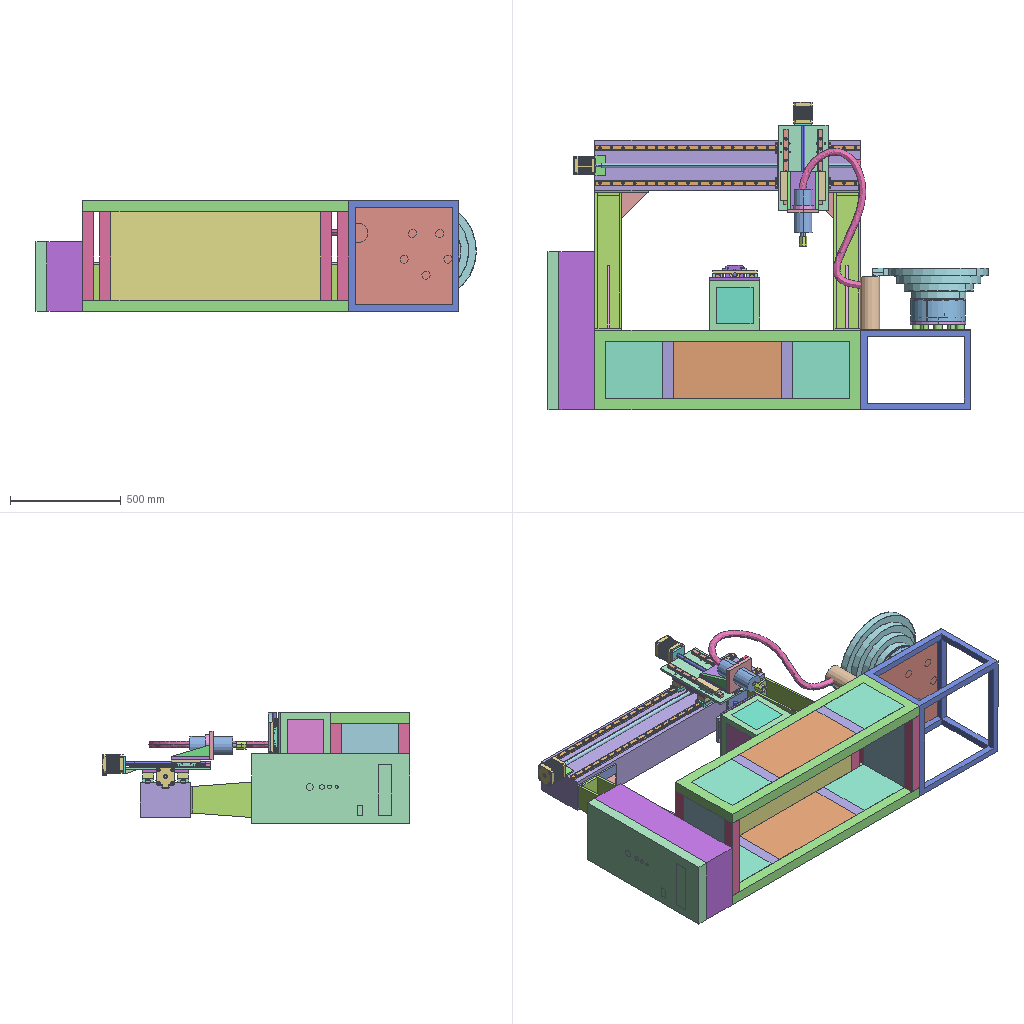Assembly | STEP file | 61 different items | 143 placed | box 1992 x 1390 x 500 mm
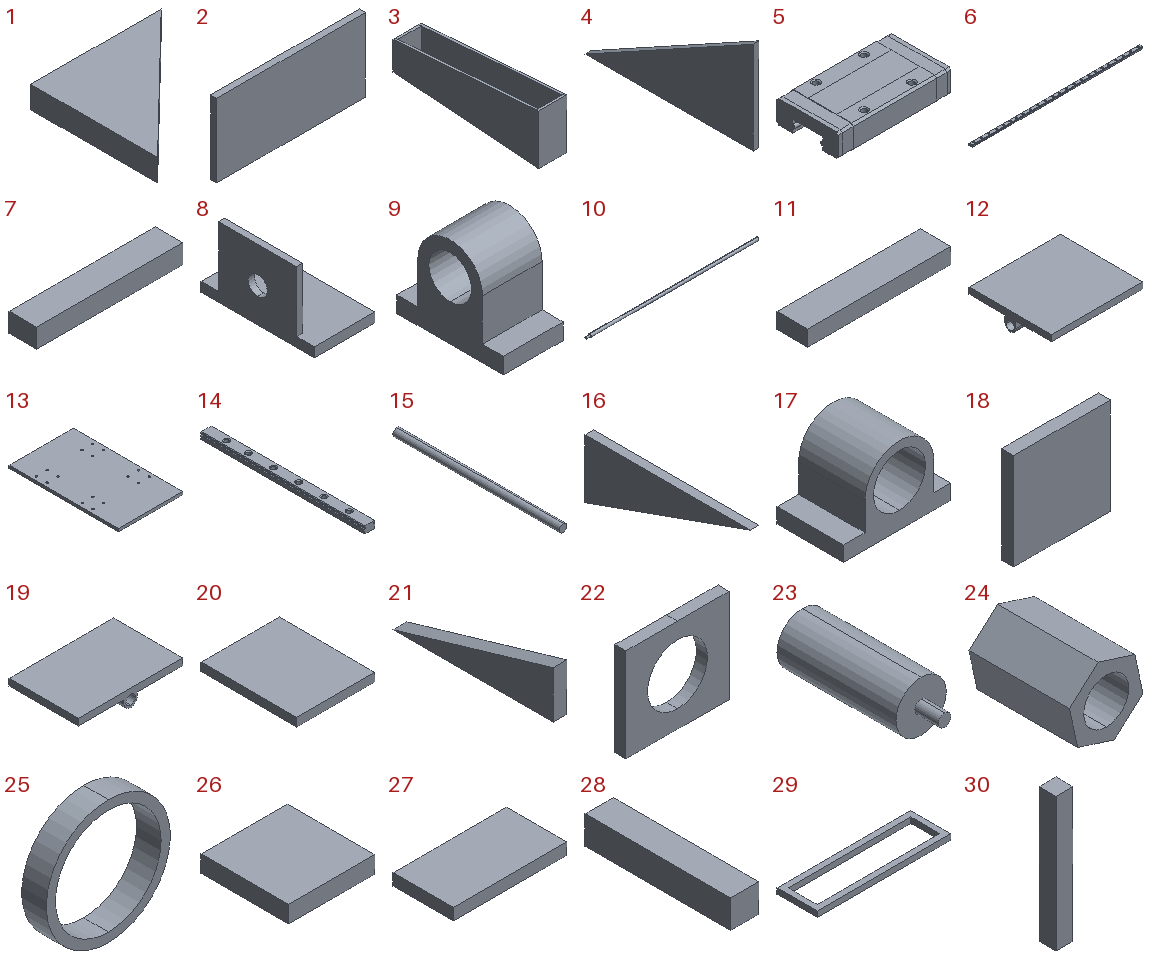Parts list (item | quantity | size | volume):
1 | x2 | 117.801 x 114.536 x 20 mm | 134925 mm3
2 | x2 | 243.554 x 10 x 120 mm | 292264 mm3
3 | x2 | 120 x 620.836 x 212.718 mm | 2999336 mm3
4 | x2 | 10 x 283.933 x 156.359 mm | 221977 mm3
5 | x8 | 88.2 x 48.75 x 18.375 mm | 58847 mm3
6 | x2 | 1200 x 22.5 x 15 mm | 367199 mm3
7 | x1 | 1200 x 227 x 156.72 mm | 9554357 mm3
8 | x1 | 48 x 90 x 55.597 mm | 46408 mm3
9 | x1 | 28 x 50 x 42.426 mm | 28637 mm3
10 | x1 | 1200 x 20 x 20 mm | 371431 mm3
11 | x2 | 229 x 49.201 x 25.123 mm | 283059 mm3
12 | x1 | 229 x 206.363 x 45.369 mm | 819761 mm3
13 | x1 | 225.075 x 384.491 x 10 mm | 860870 mm3
14 | x4 | 22.5 x 340 x 15 mm | 104637 mm3
15 | x2 | 18 x 384.491 x 18 mm | 97841 mm3
16 | x2 | 3 x 56.217 x 20 mm | 1687 mm3
17 | x1 | 37.23 x 23 x 26.824 mm | 9039 mm3
18 | x1 | 77.948 x 9.733 x 78 mm | 59173 mm3
19 | x2 | 200.887 x 133 x 32.213 mm | 365729 mm3
20 | x1 | 140.887 x 173 x 15 mm | 365603 mm3
21 | x2 | 15 x 173 x 50.952 mm | 66110 mm3
22 | x1 | 140.887 x 15 x 127.87 mm | 191936 mm3
23 | x1 | 81.521 x 231.5 x 81.521 mm | 1019717 mm3
24 | x1 | 32.935 x 45 x 33.783 mm | 20505 mm3
25 | x1 | 95.525 x 19 x 95.525 mm | 36998 mm3
26 | x4 | 255.311 x 259.164 x 50 mm | 3308367 mm3
27 | x2 | 489.379 x 259.164 x 50 mm | 6341468 mm3
28 | x4 | 50 x 259.164 x 50 mm | 647910 mm3
29 | x2 | 1200 x 359.164 x 50 mm | 7295820 mm3
30 | x6 | 50 x 50 x 400 mm | 1000000 mm3
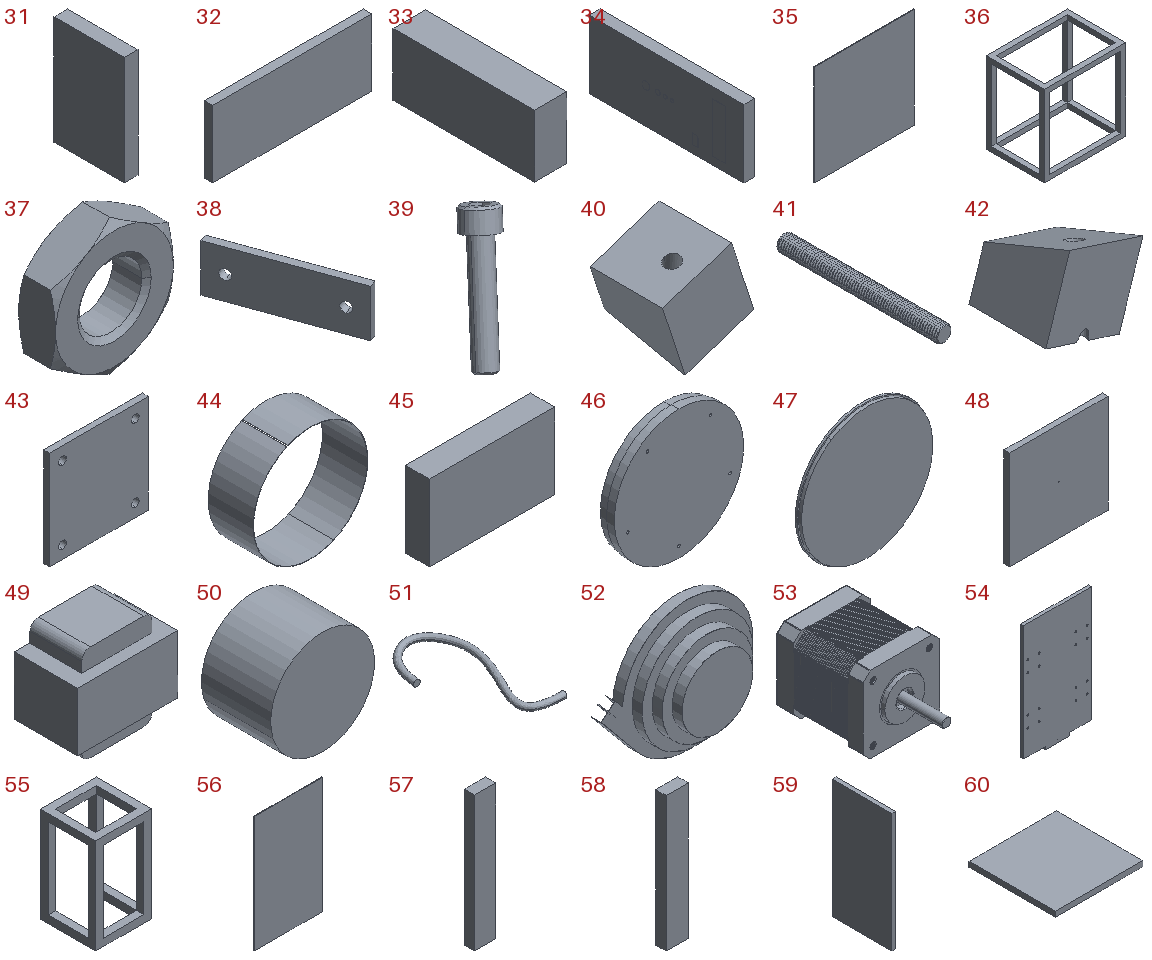31 | x2 | 50 x 259.164 x 400 mm | 5183281 mm3
32 | x1 | 947.9 x 50 x 400 mm | 18958001 mm3
33 | x1 | 162.496 x 714.237 x 313.918 mm | 36433685 mm3
34 | x1 | 51.504 x 714.237 x 313.918 mm | 11131790 mm3
35 | x1 | 498.959 x 2 x 500 mm | 498959 mm3
36 | x1 | 498.959 x 359.164 x 500 mm | 4457242 mm3
37 | x12 | 7.84 x 2.45 x 9.053 mm | 94.615 mm3
38 | x10 | 27.146 x 65.804 x 24.5 mm | 6425 mm3
39 | x10 | 14.373 x 15.735 x 28.731 mm | 656.353 mm3
40 | x5 | 30.872 x 24.5 x 30.872 mm | 11634 mm3
41 | x4 | 4.9 x 49 x 4.9 mm | 811.939 mm3
42 | x5 | 30.872 x 24.5 x 30.872 mm | 11423 mm3
43 | x1 | 66.15 x 3.92 x 66.15 mm | 16827 mm3
44 | x1 | 246.568 x 97.02 x 246.568 mm | 58546 mm3
45 | x1 | 58.8 x 11.27 x 35.77 mm | 23704 mm3
46 | x1 | 249.9 x 29.4 x 249.9 mm | 1411943 mm3
47 | x1 | 249.9 x 9.8 x 249.9 mm | 469473 mm3
48 | x1 | 61.25 x 3.43 x 61.25 mm | 12867 mm3
49 | x1 | 58.8 x 37.24 x 56.35 mm | 101666 mm3
50 | x5 | 36.75 x 34.3 x 36.75 mm | 26254 mm3
51 | x1 | 324.826 x 634.125 x 30 mm | 760478 mm3
52 | x1 | 524.053 x 137.2 x 450.8 mm | 389951 mm3
53 | x3 | 84 x 145 x 94 mm | 649991 mm3
54 | x1 | 225.075 x 66.921 x 394.223 mm | 895884 mm3
55 | x1 | 226.259 x 224 x 387.57 mm | 2434549 mm3
56 | x1 | 226.259 x 2 x 387.57 mm | 175382 mm3
57 | x1 | 20.737 x 10 x 133 mm | 27580 mm3
58 | x1 | 21.772 x 10 x 133 mm | 28956 mm3
59 | x2 | 10 x 164 x 327.57 mm | 537214 mm3
60 | x2 | 166.259 x 164 x 10 mm | 272664 mm3
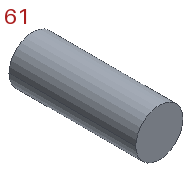61 | x1 | 89.417 x 240 x 89.417 mm | 636634 mm3
Placements (level | parent | child | x y z in mm | rotation matrix by rows):
1 | subassembly 2 | subassembly 3 | -0.0 -0.0 -0.0 | 1 0 0 0 1 0 0 0 1
1 | subassembly 2 | subassembly 3 | -0.0 -0.0 -0.0 | -1 0 0 0 1 0 0 0 -1
1 | subassembly 2 | subassembly 4 | -0.0 -0.0 -0.0 | 1 0 0 0 1 0 0 0 1
1 | subassembly 2 | subassembly 4 | 0.0 870.0 0.0 | -1 0 0 0 -1 0 0 0 1
1 | subassembly 2 | subassembly 5 | -0.0 -0.0 -0.0 | 1 0 0 0 1 0 0 0 1
1 | subassembly 2 | subassembly 5 | 1080.0 -0.0 -0.0 | 1 0 0 0 1 0 0 0 1
1 | subassembly 2 | subassembly 6 | -0.0 -0.0 -0.0 | 1 0 0 0 1 0 0 0 1
1 | subassembly 2 | subassembly 6 | 1077.681 0.0 0.0 | 1 0 0 0 1 0 0 0 1
1 | subassembly 2 | subassembly 7 | -0.0 -0.0 -0.0 | 1 0 0 0 1 0 0 0 1
1 | subassembly 2 | subassembly 7 | 841.273 1107.0 -0.0 | -1 0 0 0 -1 0 0 0 1
1 | subassembly 2 | subassembly 7 | -159.975 -0.0 -0.0 | 1 0 0 0 1 0 0 0 1
1 | subassembly 2 | subassembly 7 | 681.297 1107.0 -0.0 | -1 0 0 0 -1 0 0 0 1
1 | subassembly 2 | subassembly 7 | 896.886 38.582 71.806 | 0 -1 0 1 0 0 0 0 1
1 | subassembly 2 | subassembly 7 | -215.589 879.855 71.806 | 0 1 0 -1 0 0 0 0 1
1 | subassembly 2 | subassembly 7 | 588.111 -30.042 705.358 | 0 -1 0 0 0 1 -1 0 -0
1 | subassembly 2 | subassembly 7 | -524.365 -30.042 -135.915 | 0 1 0 0 0 1 1 0 -0
1 | subassembly 2 | subassembly 8 | -0.0 -0.0 -0.0 | 1 0 0 0 1 0 0 0 1
1 | subassembly 2 | subassembly 8 | -0.0 1107.0 -0.0 | -1 0 0 0 -1 0 0 0 1
1 | subassembly 2 | subassembly 9 | -0.0 -0.0 -0.0 | 1 0 0 0 1 0 0 0 1
1 | subassembly 2 | subassembly 10 | -0.0 -0.0 -0.0 | 1 0 0 0 1 0 0 0 1
1 | subassembly 2 | subassembly 11 | -0.0 -0.0 -0.0 | 1 0 0 0 1 0 0 0 1
1 | subassembly 2 | subassembly 12 | -0.0 -0.0 -0.0 | 1 0 0 0 1 0 0 0 1
1 | subassembly 2 | subassembly 13 | -0.0 -0.0 -0.0 | 1 0 0 0 1 0 0 0 1
1 | subassembly 2 | subassembly 13 | -0.0 157.162 -0.0 | 1 0 0 0 1 0 0 0 1
1 | subassembly 2 | subassembly 14 | -0.0 -0.0 -0.0 | 1 0 0 0 1 0 0 0 1
1 | subassembly 2 | subassembly 15 | -0.0 -0.0 -0.0 | 1 0 0 0 1 0 0 0 1
1 | subassembly 2 | subassembly 16 | -0.0 -0.0 -0.0 | 1 0 0 0 1 0 0 0 1
1 | subassembly 2 | subassembly 16 | 155.137 -0.0 0.0 | 1 0 0 0 1 0 0 0 1
1 | subassembly 2 | subassembly 16 | -308.776 -101.849 743.94 | 1 0 0 0 0 1 0 -1 0
1 | subassembly 2 | subassembly 16 | -153.638 -101.849 743.94 | 1 0 0 0 0 1 0 -1 -0
1 | subassembly 2 | subassembly 17 | -0.0 -0.0 -0.0 | 1 0 0 0 1 0 0 0 1
1 | subassembly 2 | subassembly 17 | 372.522 222.018 743.94 | -1 0 0 0 0 -1 0 -1 0
1 | subassembly 2 | subassembly 18 | -0.0 -0.0 -0.0 | 1 0 0 0 1 0 0 0 1
1 | subassembly 2 | subassembly 18 | -44.948 0.0 -0.0 | 1 0 0 0 1 0 0 0 1
1 | subassembly 2 | subassembly 19 | -0.0 -0.0 -0.0 | 1 0 0 0 1 0 0 0 1
1 | subassembly 2 | subassembly 20 | -0.0 -0.0 -0.0 | 1 0 0 0 1 0 0 0 1
1 | subassembly 2 | subassembly 21 | -0.0 -0.0 -0.0 | 1 0 0 0 1 0 0 0 1
1 | subassembly 2 | subassembly 21 | -308.776 -101.849 743.94 | 1 0 0 0 0 1 0 -1 0
1 | subassembly 2 | subassembly 22 | -0.0 -0.0 -0.0 | 1 0 0 0 1 0 0 0 1
1 | subassembly 2 | subassembly 23 | -0.0 -0.0 -0.0 | 1 0 0 0 1 0 0 0 1
1 | subassembly 2 | subassembly 23 | 125.887 -0.0 0.0 | 1 0 0 0 1 0 0 0 1
1 | subassembly 2 | subassembly 24 | -0.0 -0.0 -0.0 | 1 0 0 0 1 0 0 0 1
1 | subassembly 2 | subassembly 25 | -0.0 -0.0 -0.0 | 1 0 0 0 1 0 0 0 1
1 | subassembly 2 | subassembly 26 | -0.0 -0.0 -0.0 | 1 0 0 0 1 0 0 0 1
1 | subassembly 2 | subassembly 27 | -0.0 -0.0 -0.0 | 1 0 0 0 1 0 0 0 1
1 | subassembly 2 | subassembly 28 | -0.0 -0.0 -0.0 | 1 0 0 0 1 0 0 0 1
1 | subassembly 2 | subassembly 28 | 844.689 -0.0 -0.0 | 1 0 0 0 1 0 0 0 1
1 | subassembly 2 | subassembly 28 | 844.689 -0.0 -450.0 | 1 0 0 0 1 0 0 0 1
1 | subassembly 2 | subassembly 28 | -0.0 -0.0 -450.0 | 1 0 0 0 1 0 0 0 1
1 | subassembly 2 | subassembly 29 | -0.0 -0.0 -0.0 | 1 0 0 0 1 0 0 0 1
1 | subassembly 2 | subassembly 29 | -0.0 -0.0 -450.0 | 1 0 0 0 1 0 0 0 1
1 | subassembly 2 | subassembly 30 | -0.0 -0.0 -0.0 | 1 0 0 0 1 0 0 0 1
1 | subassembly 2 | subassembly 30 | 0.0 -0.0 737.282 | -1 0 0 0 1 0 0 0 -1
1 | subassembly 2 | subassembly 30 | -0.0 -0.0 -450.0 | 1 0 0 0 1 0 0 0 1
1 | subassembly 2 | subassembly 30 | 0.0 0.0 287.282 | -1 0 0 0 1 0 0 0 -1
1 | subassembly 2 | subassembly 31 | -0.0 -0.0 -0.0 | 1 0 0 0 1 0 0 0 1
1 | subassembly 2 | subassembly 31 | 0.0 0.0 -450.0 | 1 0 0 0 1 0 0 0 1
1 | subassembly 2 | subassembly 32 | -0.0 -0.0 -0.0 | 1 0 0 0 1 0 0 0 1
1 | subassembly 2 | subassembly 32 | -76.05 -0.0 -0.0 | 1 0 0 0 1 0 0 0 1
1 | subassembly 2 | subassembly 32 | -76.05 -309.164 -0.0 | 1 0 0 0 1 0 0 0 1
1 | subassembly 2 | subassembly 32 | 997.9 0.0 -0.0 | 1 0 0 0 1 0 0 0 1
1 | subassembly 2 | subassembly 32 | 1073.95 0.0 -0.0 | 1 0 0 0 1 0 0 0 1
1 | subassembly 2 | subassembly 32 | 76.05 -309.164 287.282 | -1 0 0 0 1 0 0 0 -1
1 | subassembly 2 | subassembly 33 | -0.0 -0.0 -0.0 | 1 0 0 0 1 0 0 0 1
1 | subassembly 2 | subassembly 33 | 1150.0 0.0 0.0 | 1 0 0 0 1 0 0 0 1
1 | subassembly 2 | subassembly 34 | -0.0 -0.0 -0.0 | 1 0 0 0 1 0 0 0 1
1 | subassembly 2 | subassembly 35 | -0.0 -0.0 -0.0 | 1 0 0 0 1 0 0 0 1
1 | subassembly 2 | subassembly 36 | -0.0 -0.0 -0.0 | 1 0 0 0 1 0 0 0 1
1 | subassembly 2 | subassembly 37 | -0.0 -0.0 -0.0 | 1 0 0 0 1 0 0 0 1
1 | subassembly 2 | subassembly 38 | -0.0 -0.0 -0.0 | 1 0 0 0 1 0 0 0 1
1 | subassembly 2 | subassembly 39 | -0.0 -0.0 -0.0 | 1 0 0 0 1 0 0 0 1
1 | subassembly 2 | subassembly 39 | 0.0001 -6.37 48.999 | 1 0 0 0 1 0 0 0 1
1 | subassembly 2 | subassembly 39 | -49.0 -6.37 -0.0001 | 1 0 0 0 1 0 0 0 1
1 | subassembly 2 | subassembly 39 | -49.0 -23.462 49 | 1 0 0 0 1 0 0 0 1
1 | subassembly 2 | subassembly 39 | -49 0.0 48.999 | 1 0 -1e-06 0 1 0 1e-06 0 1
1 | subassembly 2 | subassembly 39 | -49 -6.37 49.001 | 1 0 0 0 1 0 0 0 1
1 | subassembly 2 | subassembly 39 | 0.0 -23.462 -0.0001 | 1 0 0 0 1 0 0 0 1
1 | subassembly 2 | subassembly 39 | -49.0 -23.462 -0.0002 | 1 0 0 0 1 0 0 0 1
1 | subassembly 2 | subassembly 39 | 0.0 -23.462 49.0 | 1 0 0 0 1 0 0 0 1
1 | subassembly 2 | subassembly 39 | 0.0 -6.37 -0.0 | 1 0 0 0 1 0 0 0 1
1 | subassembly 2 | subassembly 39 | -49.0 0.0 0.0001 | 1 0 0 0 1 0 0 0 1
1 | subassembly 2 | subassembly 39 | 0.0 -0.0 49 | 1 0 0 0 1 0 0 0 1
1 | subassembly 2 | subassembly 40 | -0.0 -0.0 -0.0 | 1 0 0 0 1 0 0 0 1
1 | subassembly 2 | subassembly 40 | 808.883 -1.676 -796.145 | 0.309 0 -0.9511 0 1 0 0.9511 0 0.309
1 | subassembly 2 | subassembly 40 | 502.616 -0.0 1015.316 | 0.309 0 0.9511 0 1 0 -0.9511 0 0.309
1 | subassembly 2 | subassembly 40 | 1813.718 -0.0 -265.789 | -0.809 0 -0.5878 0 1 0 0.5878 0 -0.809
1 | subassembly 2 | subassembly 40 | 1817.444 -1.676 -268.495 | -0.809 0 -0.5878 0 1 0 0.5878 0 -0.809
1 | subassembly 2 | subassembly 40 | 1623.556 -0.0 851.049 | -0.809 0 0.5878 0 1 0 -0.5878 0 -0.809
1 | subassembly 2 | subassembly 40 | 1627.281 -1.676 853.756 | -0.809 0 0.5878 0 1 0 -0.5878 0 -0.809
1 | subassembly 2 | subassembly 40 | -4.604 -1.676 -0.0 | 1 0 0 0 1 0 0 0 1
1 | subassembly 2 | subassembly 40 | 810.306 -0.0 -791.766 | 0.309 0 -0.9511 0 1 0 0.9511 0 0.309
1 | subassembly 2 | subassembly 40 | 501.193 -1.676 1019.695 | 0.309 0 0.9511 0 1 0 -0.9511 0 0.309
1 | subassembly 2 | subassembly 41 | -0.0 -0.0 -0.0 | 1 0 0 0 1 0 0 0 1
1 | subassembly 2 | subassembly 41 | 1057.854 -661.138 -476.93 | -0.1707 -0.9797 0.1055 0.7998 -0.2002 -0.5659 0.5755 -0.01224 0.8177
1 | subassembly 2 | subassembly 41 | 362.365 -707.182 -147.994 | 0.4946 -0.3144 0.8102 0.7998 -0.2002 -0.5659 0.3402 0.9279 0.1524
1 | subassembly 2 | subassembly 41 | 485.857 46.045 1015.316 | 0.309 0 0.9511 0 1 0 -0.9511 0 0.309
1 | subassembly 2 | subassembly 41 | 487.401 -661.138 615.103 | 0.4764 0.7854 0.3953 0.7998 -0.2002 -0.5659 -0.3653 0.5857 -0.7235
1 | subassembly 2 | subassembly 41 | 375.924 -661.138 -138.143 | 0.4946 -0.3144 0.8102 0.7998 -0.2002 -0.5659 0.3402 0.9279 0.1524
1 | subassembly 2 | subassembly 41 | 502.616 -0.0 1015.316 | 0.309 0 0.9511 0 1 0 -0.9511 0 0.309
1 | subassembly 2 | subassembly 41 | -5.179 46.045 -15.939 | 1 0 0 0 1 0 0 0 1
1 | subassembly 2 | subassembly 41 | 1063.033 -707.182 -492.869 | -0.1707 -0.9797 0.1055 0.7998 -0.2002 -0.5659 0.5755 -0.01224 0.8177
1 | subassembly 2 | subassembly 41 | 473.843 -707.182 624.953 | 0.4764 0.7854 0.3953 0.7998 -0.2002 -0.5659 -0.3653 0.5857 -0.7235
1 | subassembly 2 | subassembly 42 | -0.0 -0.0 -0.0 | 1 0 0 0 1 0 0 0 1
1 | subassembly 2 | subassembly 42 | 810.306 -0.0 -791.766 | 0.309 0 -0.9511 0 1 0 0.9511 0 0.309
1 | subassembly 2 | subassembly 42 | 1813.718 0.0 -265.789 | -0.809 0 -0.5878 0 1 0 0.5878 0 -0.809
1 | subassembly 2 | subassembly 42 | 502.616 -0.0 1015.316 | 0.309 0 0.9511 0 1 0 -0.9511 0 0.309
1 | subassembly 2 | subassembly 42 | 1623.556 -0.0 851.049 | -0.809 0 0.5878 0 1 0 -0.5878 0 -0.809
1 | subassembly 2 | subassembly 43 | -0.0 -0.0 -0.0 | 1 0 0 0 1 0 0 0 1
1 | subassembly 2 | subassembly 43 | -49.0 0.0 -49.0 | 1 0 0 0 1 0 0 0 1
1 | subassembly 2 | subassembly 43 | -0.0 -0.0 -49.0 | 1 0 0 0 1 0 0 0 1
1 | subassembly 2 | subassembly 43 | -49.0 0.0 -0.0 | 1 0 0 0 1 0 0 0 1
1 | subassembly 2 | subassembly 44 | -0.0 -0.0 -0.0 | 1 0 0 0 1 0 0 0 1
1 | subassembly 2 | subassembly 44 | 502.616 -0.0 1015.316 | 0.309 0 0.9511 0 1 0 -0.9511 0 0.309
1 | subassembly 2 | subassembly 44 | 1623.556 -0.0 851.049 | -0.809 0 0.5878 0 1 0 -0.5878 0 -0.809
1 | subassembly 2 | subassembly 44 | 810.306 -0.0 -791.766 | 0.309 0 -0.9511 0 1 0 0.9511 0 0.309
1 | subassembly 2 | subassembly 44 | 1813.718 -0.0 -265.789 | -0.809 0 -0.5878 0 1 0 0.5878 0 -0.809
1 | subassembly 2 | subassembly 45 | -0.0 -0.0 -0.0 | 1 0 0 0 1 0 0 0 1
1 | subassembly 2 | subassembly 46 | -0.0 -0.0 -0.0 | 1 0 0 0 1 0 0 0 1
1 | subassembly 2 | subassembly 47 | -0.0 -0.0 -0.0 | 1 0 0 0 1 0 0 0 1
1 | subassembly 2 | subassembly 48 | -0.0 -0.0 -0.0 | 1 0 0 0 1 0 0 0 1
1 | subassembly 2 | subassembly 49 | -0.0 -0.0 -0.0 | 1 0 0 0 1 0 0 0 1
1 | subassembly 2 | subassembly 50 | -0.0 -0.0 -0.0 | 1 0 0 0 1 0 0 0 1
1 | subassembly 2 | subassembly 51 | -0.0 -0.0 -0.0 | 1 0 0 0 1 0 0 0 1
1 | subassembly 2 | subassembly 52 | -0.0 -0.0 -0.0 | 1 0 0 0 1 0 0 0 1
1 | subassembly 2 | subassembly 52 | 759.25 -0.0 1097.011 | 0 0 1 0 1 0 -1 0 -0
1 | subassembly 2 | subassembly 52 | 99.029 -0.0 -71.949 | 1 0 0 0 1 0 0 0 1
1 | subassembly 2 | subassembly 52 | 881.657 0.0 1097.011 | 0 0 1 0 1 0 -1 0 -0
1 | subassembly 2 | subassembly 52 | 198.058 -0.0 -0.0 | 1 0 0 0 1 0 0 0 1
1 | subassembly 2 | subassembly 53 | -0.0 -0.0 -0.0 | 1 0 0 0 1 0 0 0 1
1 | subassembly 2 | subassembly 54 | -0.0 -0.0 -0.0 | 1 0 0 0 1 0 0 0 1
1 | subassembly 2 | subassembly 55 | -0.0 -0.0 -0.0 | 1 0 0 0 1 0 0 0 1
1 | subassembly 2 | subassembly 55 | 144.522 212.851 -57.028 | 0 -1 0 1 0 0 0 0 1
1 | subassembly 2 | subassembly 55 | -308.776 -101.849 743.94 | 1 0 0 0 0 1 0 -1 0
1 | subassembly 2 | subassembly 56 | -0.0 -0.0 -0.0 | 1 0 0 0 1 0 0 0 1
1 | subassembly 2 | subassembly 57 | -0.0 -0.0 -0.0 | 1 0 0 0 1 0 0 0 1
1 | subassembly 2 | subassembly 58 | -0.0 -0.0 -0.0 | 1 0 0 0 1 0 0 0 1
1 | subassembly 2 | subassembly 59 | -0.0 -0.0 -0.0 | 1 0 0 0 1 0 0 0 1
1 | subassembly 2 | subassembly 60 | -0.0 -0.0 -0.0 | 1 0 0 0 1 0 0 0 1
1 | subassembly 2 | subassembly 61 | -0.0 -0.0 -0.0 | 1 0 0 0 1 0 0 0 1
1 | subassembly 2 | subassembly 61 | 216.259 0.0 -0.0 | 1 0 0 0 1 0 0 0 1
1 | subassembly 2 | subassembly 62 | -0.0 -0.0 -0.0 | 1 0 0 0 1 0 0 0 1
1 | subassembly 2 | subassembly 62 | -0.0 -0.0 -377.57 | 1 0 0 0 1 0 0 0 1
1 | subassembly 2 | subassembly 63 | -0.0 -0.0 -0.0 | 1 0 0 0 1 0 0 0 1